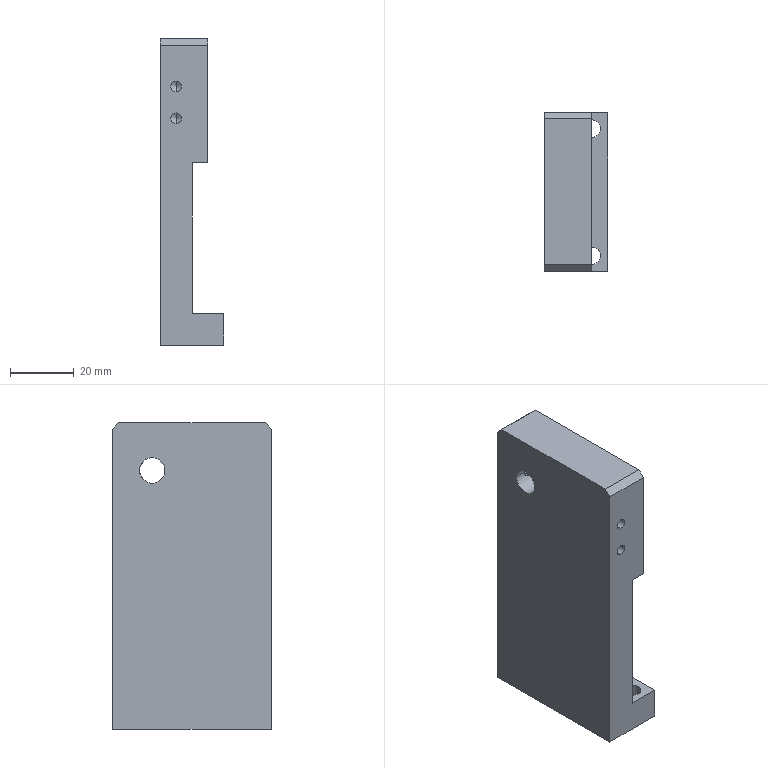Part | STEP file | 11-FG-B00911 | 1 solid | 32 faces | box 20 x 50 x 96.4 mm | volume 61320 mm3 | cylinder 14 | plane 12 | cone 6 | commonest cylinder face diameters 3.3 x8 5.5 x4 8 x2
STEP:
#1=CARTESIAN_POINT('',(17.75,5.,-7.4));
#2=VERTEX_POINT('',#1);
#3=CARTESIAN_POINT('',(12.25,5.,-7.4));
#4=VERTEX_POINT('',#3);
#5=CARTESIAN_POINT('',(15.,5.,-7.4));
#6=DIRECTION('',(0.,0.,-1.));
#7=DIRECTION('',(1.,0.,0.));
#8=AXIS2_PLACEMENT_3D('',#5,#6,#7);
#9=CIRCLE('',#8,2.75);
#10=EDGE_CURVE('',#2,#4,#9,.T.);
#11=ORIENTED_EDGE('',*,*,#10,.T.);
#12=CARTESIAN_POINT('',(12.25,5.,2.6));
#13=VERTEX_POINT('',#12);
#14=CARTESIAN_POINT('',(12.25,5.,-7.4));
#15=DIRECTION('',(0.,0.,1.));
#16=VECTOR('',#15,1000.);
#17=LINE('',#14,#16);
#18=EDGE_CURVE('',#4,#13,#17,.T.);
#19=ORIENTED_EDGE('',*,*,#18,.T.);
#20=CARTESIAN_POINT('',(17.75,5.,2.6));
#21=VERTEX_POINT('',#20);
#22=CARTESIAN_POINT('',(15.,5.,2.6));
#23=DIRECTION('',(0.,0.,1.));
#24=DIRECTION('',(-1.,0.,0.));
#25=AXIS2_PLACEMENT_3D('',#22,#23,#24);
#26=CIRCLE('',#25,2.75);
#27=EDGE_CURVE('',#13,#21,#26,.T.);
#28=ORIENTED_EDGE('',*,*,#27,.T.);
#29=CARTESIAN_POINT('',(17.75,5.,-7.4));
#30=DIRECTION('',(0.,0.,1.));
#31=VECTOR('',#30,1000.);
#32=LINE('',#29,#31);
#33=EDGE_CURVE('',#2,#21,#32,.T.);
#34=ORIENTED_EDGE('',*,*,#33,.F.);
#35=EDGE_LOOP('',(#11,#19,#28,#34));
#36=FACE_OUTER_BOUND('',#35,.T.);
#37=CARTESIAN_POINT('',(15.,5.,-7.4));
#38=DIRECTION('',(0.,0.,1.));
#39=DIRECTION('',(1.,0.,0.));
#40=AXIS2_PLACEMENT_3D('',#37,#38,#39);
#41=CYLINDRICAL_SURFACE('',#40,2.75);
#42=ADVANCED_FACE('',(#36),#41,.F.);
#43=CARTESIAN_POINT('',(5.,10.1,65.65));
#44=VERTEX_POINT('',#43);
#45=CARTESIAN_POINT('',(5.,10.1,62.35));
#46=VERTEX_POINT('',#45);
#47=CARTESIAN_POINT('',(5.,10.1,64.));
#48=DIRECTION('',(0.,-1.,0.));
#49=DIRECTION('',(0.,0.,-1.));
#50=AXIS2_PLACEMENT_3D('',#47,#48,#49);
#51=CIRCLE('',#50,1.65);
#52=EDGE_CURVE('',#44,#46,#51,.T.);
#53=ORIENTED_EDGE('',*,*,#52,.F.);
#54=CARTESIAN_POINT('',(5.,0.,65.65));
#55=VERTEX_POINT('',#54);
#56=CARTESIAN_POINT('',(5.,0.,65.65));
#57=DIRECTION('',(0.,-1.,0.));
#58=VECTOR('',#57,1000.);
#59=LINE('',#56,#58);
#60=EDGE_CURVE('',#44,#55,#59,.T.);
#61=ORIENTED_EDGE('',*,*,#60,.T.);
#62=CARTESIAN_POINT('',(5.,0.,62.35));
#63=VERTEX_POINT('',#62);
#64=CARTESIAN_POINT('',(5.,0.,64.));
#65=DIRECTION('',(0.,-1.,0.));
#66=DIRECTION('',(0.,0.,-1.));
#67=AXIS2_PLACEMENT_3D('',#64,#65,#66);
#68=CIRCLE('',#67,1.65);
#69=EDGE_CURVE('',#55,#63,#68,.T.);
#70=ORIENTED_EDGE('',*,*,#69,.T.);
#71=CARTESIAN_POINT('',(5.,0.,62.35));
#72=DIRECTION('',(0.,-1.,0.));
#73=VECTOR('',#72,1000.);
#74=LINE('',#71,#73);
#75=EDGE_CURVE('',#46,#63,#74,.T.);
#76=ORIENTED_EDGE('',*,*,#75,.F.);
#77=EDGE_LOOP('',(#53,#61,#70,#76));
#78=FACE_OUTER_BOUND('',#77,.T.);
#79=CARTESIAN_POINT('',(5.,0.,64.));
#80=DIRECTION('',(0.,-1.,0.));
#81=DIRECTION('',(0.,0.,-1.));
#82=AXIS2_PLACEMENT_3D('',#79,#80,#81);
#83=CYLINDRICAL_SURFACE('',#82,1.65);
#84=ADVANCED_FACE('',(#78),#83,.F.);
#85=CARTESIAN_POINT('',(5.,11.091,64.));
#86=VERTEX_POINT('',#85);
#87=CARTESIAN_POINT('',(5.,10.1,62.35));
#88=DIRECTION('',(0.,-0.515,-0.8572));
#89=VECTOR('',#88,1000.);
#90=LINE('',#87,#89);
#91=EDGE_CURVE('',#86,#46,#90,.T.);
#92=ORIENTED_EDGE('',*,*,#91,.F.);
#93=CARTESIAN_POINT('',(5.,10.1,65.65));
#94=DIRECTION('',(0.,-0.515,0.8572));
#95=VECTOR('',#94,1000.);
#96=LINE('',#93,#95);
#97=EDGE_CURVE('',#86,#44,#96,.T.);
#98=ORIENTED_EDGE('',*,*,#97,.T.);
#99=ORIENTED_EDGE('',*,*,#52,.T.);
#100=EDGE_LOOP('',(#92,#98,#99));
#101=FACE_OUTER_BOUND('',#100,.T.);
#102=CARTESIAN_POINT('',(5.,10.1,64.));
#103=DIRECTION('',(0.,-1.,0.));
#104=DIRECTION('',(0.,0.,-1.));
#105=AXIS2_PLACEMENT_3D('',#102,#103,#104);
#106=CONICAL_SURFACE('',#105,1.65,1.03);
#107=ADVANCED_FACE('',(#101),#106,.F.);
#108=CARTESIAN_POINT('',(5.,10.1,75.65));
#109=VERTEX_POINT('',#108);
#110=CARTESIAN_POINT('',(5.,10.1,72.35));
#111=VERTEX_POINT('',#110);
#112=CARTESIAN_POINT('',(5.,10.1,74.));
#113=DIRECTION('',(0.,-1.,0.));
#114=DIRECTION('',(0.,0.,-1.));
#115=AXIS2_PLACEMENT_3D('',#112,#113,#114);
#116=CIRCLE('',#115,1.65);
#117=EDGE_CURVE('',#109,#111,#116,.T.);
#118=ORIENTED_EDGE('',*,*,#117,.F.);
#119=CARTESIAN_POINT('',(5.,0.,75.65));
#120=VERTEX_POINT('',#119);
#121=CARTESIAN_POINT('',(5.,0.,75.65));
#122=DIRECTION('',(0.,-1.,0.));
#123=VECTOR('',#122,1000.);
#124=LINE('',#121,#123);
#125=EDGE_CURVE('',#109,#120,#124,.T.);
#126=ORIENTED_EDGE('',*,*,#125,.T.);
#127=CARTESIAN_POINT('',(5.,0.,72.35));
#128=VERTEX_POINT('',#127);
#129=CARTESIAN_POINT('',(5.,0.,74.));
#130=DIRECTION('',(0.,-1.,0.));
#131=DIRECTION('',(0.,0.,-1.));
#132=AXIS2_PLACEMENT_3D('',#129,#130,#131);
#133=CIRCLE('',#132,1.65);
#134=EDGE_CURVE('',#120,#128,#133,.T.);
#135=ORIENTED_EDGE('',*,*,#134,.T.);
#136=CARTESIAN_POINT('',(5.,0.,72.35));
#137=DIRECTION('',(0.,-1.,0.));
#138=VECTOR('',#137,1000.);
#139=LINE('',#136,#138);
#140=EDGE_CURVE('',#111,#128,#139,.T.);
#141=ORIENTED_EDGE('',*,*,#140,.F.);
#142=EDGE_LOOP('',(#118,#126,#135,#141));
#143=FACE_OUTER_BOUND('',#142,.T.);
#144=CARTESIAN_POINT('',(5.,0.,74.));
#145=DIRECTION('',(0.,-1.,0.));
#146=DIRECTION('',(0.,0.,-1.));
#147=AXIS2_PLACEMENT_3D('',#144,#145,#146);
#148=CYLINDRICAL_SURFACE('',#147,1.65);
#149=ADVANCED_FACE('',(#143),#148,.F.);
#150=CARTESIAN_POINT('',(5.,11.091,74.));
#151=VERTEX_POINT('',#150);
#152=CARTESIAN_POINT('',(5.,10.1,72.35));
#153=DIRECTION('',(0.,-0.515,-0.8572));
#154=VECTOR('',#153,1000.);
#155=LINE('',#152,#154);
#156=EDGE_CURVE('',#151,#111,#155,.T.);
#157=ORIENTED_EDGE('',*,*,#156,.F.);
#158=CARTESIAN_POINT('',(5.,10.1,75.65));
#159=DIRECTION('',(0.,-0.515,0.8572));
#160=VECTOR('',#159,1000.);
#161=LINE('',#158,#160);
#162=EDGE_CURVE('',#151,#109,#161,.T.);
#163=ORIENTED_EDGE('',*,*,#162,.T.);
#164=ORIENTED_EDGE('',*,*,#117,.T.);
#165=EDGE_LOOP('',(#157,#163,#164));
#166=FACE_OUTER_BOUND('',#165,.T.);
#167=CARTESIAN_POINT('',(5.,10.1,74.));
#168=DIRECTION('',(0.,-1.,0.));
#169=DIRECTION('',(0.,0.,-1.));
#170=AXIS2_PLACEMENT_3D('',#167,#168,#169);
#171=CONICAL_SURFACE('',#170,1.65,1.03);
#172=ADVANCED_FACE('',(#166),#171,.F.);
#173=CARTESIAN_POINT('',(12.25,45.,-7.4));
#174=VERTEX_POINT('',#173);
#175=CARTESIAN_POINT('',(17.75,45.,-7.4));
#176=VERTEX_POINT('',#175);
#177=CARTESIAN_POINT('',(15.,45.,-7.4));
#178=DIRECTION('',(0.,0.,1.));
#179=DIRECTION('',(1.,0.,0.));
#180=AXIS2_PLACEMENT_3D('',#177,#178,#179);
#181=CIRCLE('',#180,2.75);
#182=EDGE_CURVE('',#174,#176,#181,.T.);
#183=ORIENTED_EDGE('',*,*,#182,.F.);
#184=CARTESIAN_POINT('',(12.25,45.,2.6));
#185=VERTEX_POINT('',#184);
#186=CARTESIAN_POINT('',(12.25,45.,0.));
#187=DIRECTION('',(0.,0.,1.));
#188=VECTOR('',#187,1000.);
#189=LINE('',#186,#188);
#190=EDGE_CURVE('',#174,#185,#189,.T.);
#191=ORIENTED_EDGE('',*,*,#190,.T.);
#192=CARTESIAN_POINT('',(17.75,45.,2.6));
#193=VERTEX_POINT('',#192);
#194=CARTESIAN_POINT('',(15.,45.,2.6));
#195=DIRECTION('',(0.,0.,1.));
#196=DIRECTION('',(1.,0.,0.));
#197=AXIS2_PLACEMENT_3D('',#194,#195,#196);
#198=CIRCLE('',#197,2.75);
#199=EDGE_CURVE('',#185,#193,#198,.T.);
#200=ORIENTED_EDGE('',*,*,#199,.T.);
#201=CARTESIAN_POINT('',(17.75,45.,0.));
#202=DIRECTION('',(0.,0.,1.));
#203=VECTOR('',#202,1000.);
#204=LINE('',#201,#203);
#205=EDGE_CURVE('',#176,#193,#204,.T.);
#206=ORIENTED_EDGE('',*,*,#205,.F.);
#207=EDGE_LOOP('',(#183,#191,#200,#206));
#208=FACE_OUTER_BOUND('',#207,.T.);
#209=CARTESIAN_POINT('',(15.,45.,0.));
#210=DIRECTION('',(0.,0.,1.));
#211=DIRECTION('',(1.,0.,0.));
#212=AXIS2_PLACEMENT_3D('',#209,#210,#211);
#213=CYLINDRICAL_SURFACE('',#212,2.75);
#214=ADVANCED_FACE('',(#208),#213,.F.);
#215=CARTESIAN_POINT('',(5.,41.144,72.35));
#216=VERTEX_POINT('',#215);
#217=CARTESIAN_POINT('',(3.35,41.5,74.));
#218=VERTEX_POINT('',#217);
#219=CARTESIAN_POINT('',(5.,41.144,72.35));
#220=CARTESIAN_POINT('',(4.891,41.144,72.35));
#221=CARTESIAN_POINT('',(4.781,41.149,72.361));
#222=CARTESIAN_POINT('',(4.568,41.168,72.404));
#223=CARTESIAN_POINT('',(4.464,41.182,72.436));
#224=CARTESIAN_POINT('',(4.165,41.233,72.561));
#225=CARTESIAN_POINT('',(3.985,41.28,72.682));
#226=CARTESIAN_POINT('',(3.757,41.349,72.91));
#227=CARTESIAN_POINT('',(3.689,41.372,72.992));
#228=CARTESIAN_POINT('',(3.571,41.414,73.169));
#229=CARTESIAN_POINT('',(3.519,41.433,73.265));
#230=CARTESIAN_POINT('',(3.436,41.465,73.465));
#231=CARTESIAN_POINT('',(3.404,41.478,73.568));
#232=CARTESIAN_POINT('',(3.361,41.495,73.781));
#233=CARTESIAN_POINT('',(3.35,41.5,73.891));
#234=CARTESIAN_POINT('',(3.35,41.5,74.));
#235=B_SPLINE_CURVE_WITH_KNOTS('',3,(#219,#220,#221,#222,#223,#224,#225,#226,#227,#228,#229,#230,#231,#232,#233,#234),.UNSPECIFIED.,.F.,.F.,(4,2,2,2,2,2,2,4),(0.005217,0.005543,0.005869,0.006521,0.006847,0.007172,0.007498,0.007824),.UNSPECIFIED.);
#236=EDGE_CURVE('',#216,#218,#235,.T.);
#237=ORIENTED_EDGE('',*,*,#236,.F.);
#238=CARTESIAN_POINT('',(5.,50.,72.35));
#239=VERTEX_POINT('',#238);
#240=CARTESIAN_POINT('',(5.,50.,72.35));
#241=DIRECTION('',(0.,1.,0.));
#242=VECTOR('',#241,1000.);
#243=LINE('',#240,#242);
#244=EDGE_CURVE('',#216,#239,#243,.T.);
#245=ORIENTED_EDGE('',*,*,#244,.T.);
#246=CARTESIAN_POINT('',(5.,50.,75.65));
#247=VERTEX_POINT('',#246);
#248=CARTESIAN_POINT('',(5.,50.,74.));
#249=DIRECTION('',(0.,1.,0.));
#250=DIRECTION('',(0.,0.,1.));
#251=AXIS2_PLACEMENT_3D('',#248,#249,#250);
#252=CIRCLE('',#251,1.65);
#253=EDGE_CURVE('',#239,#247,#252,.T.);
#254=ORIENTED_EDGE('',*,*,#253,.T.);
#255=CARTESIAN_POINT('',(5.,41.144,75.65));
#256=VERTEX_POINT('',#255);
#257=CARTESIAN_POINT('',(5.,50.,75.65));
#258=DIRECTION('',(0.,1.,0.));
#259=VECTOR('',#258,1000.);
#260=LINE('',#257,#259);
#261=EDGE_CURVE('',#256,#247,#260,.T.);
#262=ORIENTED_EDGE('',*,*,#261,.F.);
#263=CARTESIAN_POINT('',(3.35,41.5,74.));
#264=CARTESIAN_POINT('',(3.35,41.5,74.218));
#265=CARTESIAN_POINT('',(3.394,41.481,74.437));
#266=CARTESIAN_POINT('',(3.519,41.433,74.735));
#267=CARTESIAN_POINT('',(3.571,41.414,74.831));
#268=CARTESIAN_POINT('',(3.69,41.372,75.009));
#269=CARTESIAN_POINT('',(3.758,41.349,75.091));
#270=CARTESIAN_POINT('',(3.909,41.303,75.243));
#271=CARTESIAN_POINT('',(3.993,41.279,75.311));
#272=CARTESIAN_POINT('',(4.17,41.236,75.43));
#273=CARTESIAN_POINT('',(4.264,41.216,75.481));
#274=CARTESIAN_POINT('',(4.565,41.164,75.607));
#275=CARTESIAN_POINT('',(4.779,41.144,75.65));
#276=CARTESIAN_POINT('',(5.,41.144,75.65));
#277=B_SPLINE_CURVE_WITH_KNOTS('',3,(#263,#264,#265,#266,#267,#268,#269,#270,#271,#272,#273,#274,#275,#276),.UNSPECIFIED.,.F.,.F.,(4,2,2,2,2,2,4),(0.007824,0.008476,0.008802,0.009127,0.009453,0.009779,0.01043),.UNSPECIFIED.);
#278=EDGE_CURVE('',#218,#256,#277,.T.);
#279=ORIENTED_EDGE('',*,*,#278,.F.);
#280=EDGE_LOOP('',(#237,#245,#254,#262,#279));
#281=FACE_OUTER_BOUND('',#280,.T.);
#282=CARTESIAN_POINT('',(5.,50.,74.));
#283=DIRECTION('',(0.,1.,0.));
#284=DIRECTION('',(0.,0.,1.));
#285=AXIS2_PLACEMENT_3D('',#282,#283,#284);
#286=CYLINDRICAL_SURFACE('',#285,1.65);
#287=ADVANCED_FACE('',(#281),#286,.F.);
#288=CARTESIAN_POINT('',(5.,39.9,62.35));
#289=VERTEX_POINT('',#288);
#290=CARTESIAN_POINT('',(5.,39.9,65.65));
#291=VERTEX_POINT('',#290);
#292=CARTESIAN_POINT('',(5.,39.9,64.));
#293=DIRECTION('',(0.,1.,0.));
#294=DIRECTION('',(0.,0.,1.));
#295=AXIS2_PLACEMENT_3D('',#292,#293,#294);
#296=CIRCLE('',#295,1.65);
#297=EDGE_CURVE('',#289,#291,#296,.T.);
#298=ORIENTED_EDGE('',*,*,#297,.F.);
#299=CARTESIAN_POINT('',(5.,50.,62.35));
#300=VERTEX_POINT('',#299);
#301=CARTESIAN_POINT('',(5.,50.,62.35));
#302=DIRECTION('',(0.,1.,0.));
#303=VECTOR('',#302,1000.);
#304=LINE('',#301,#303);
#305=EDGE_CURVE('',#289,#300,#304,.T.);
#306=ORIENTED_EDGE('',*,*,#305,.T.);
#307=CARTESIAN_POINT('',(5.,50.,65.65));
#308=VERTEX_POINT('',#307);
#309=CARTESIAN_POINT('',(5.,50.,64.));
#310=DIRECTION('',(0.,1.,0.));
#311=DIRECTION('',(0.,0.,1.));
#312=AXIS2_PLACEMENT_3D('',#309,#310,#311);
#313=CIRCLE('',#312,1.65);
#314=EDGE_CURVE('',#300,#308,#313,.T.);
#315=ORIENTED_EDGE('',*,*,#314,.T.);
#316=CARTESIAN_POINT('',(5.,50.,65.65));
#317=DIRECTION('',(0.,1.,0.));
#318=VECTOR('',#317,1000.);
#319=LINE('',#316,#318);
#320=EDGE_CURVE('',#291,#308,#319,.T.);
#321=ORIENTED_EDGE('',*,*,#320,.F.);
#322=EDGE_LOOP('',(#298,#306,#315,#321));
#323=FACE_OUTER_BOUND('',#322,.T.);
#324=CARTESIAN_POINT('',(5.,50.,64.));
#325=DIRECTION('',(0.,1.,0.));
#326=DIRECTION('',(0.,0.,1.));
#327=AXIS2_PLACEMENT_3D('',#324,#325,#326);
#328=CYLINDRICAL_SURFACE('',#327,1.65);
#329=ADVANCED_FACE('',(#323),#328,.F.);
#330=CARTESIAN_POINT('',(5.,38.909,64.));
#331=VERTEX_POINT('',#330);
#332=CARTESIAN_POINT('',(5.,39.9,65.65));
#333=DIRECTION('',(0.,0.515,0.8572));
#334=VECTOR('',#333,1000.);
#335=LINE('',#332,#334);
#336=EDGE_CURVE('',#331,#291,#335,.T.);
#337=ORIENTED_EDGE('',*,*,#336,.F.);
#338=CARTESIAN_POINT('',(5.,39.9,62.35));
#339=DIRECTION('',(0.,0.515,-0.8572));
#340=VECTOR('',#339,1000.);
#341=LINE('',#338,#340);
#342=EDGE_CURVE('',#331,#289,#341,.T.);
#343=ORIENTED_EDGE('',*,*,#342,.T.);
#344=ORIENTED_EDGE('',*,*,#297,.T.);
#345=EDGE_LOOP('',(#337,#343,#344));
#346=FACE_OUTER_BOUND('',#345,.T.);
#347=CARTESIAN_POINT('',(5.,39.9,64.));
#348=DIRECTION('',(0.,1.,0.));
#349=DIRECTION('',(0.,0.,1.));
#350=AXIS2_PLACEMENT_3D('',#347,#348,#349);
#351=CONICAL_SURFACE('',#350,1.65,1.03);
#352=ADVANCED_FACE('',(#346),#351,.F.);
#353=CARTESIAN_POINT('',(15.,41.5,74.));
#354=VERTEX_POINT('',#353);
#355=CARTESIAN_POINT('',(15.,33.5,74.));
#356=VERTEX_POINT('',#355);
#357=CARTESIAN_POINT('',(15.,37.5,74.));
#358=DIRECTION('',(-1.,0.,0.));
#359=DIRECTION('',(0.,-1.,0.));
#360=AXIS2_PLACEMENT_3D('',#357,#358,#359);
#361=CIRCLE('',#360,4.);
#362=EDGE_CURVE('',#354,#356,#361,.T.);
#363=ORIENTED_EDGE('',*,*,#362,.F.);
#364=CARTESIAN_POINT('',(6.65,41.5,74.));
#365=VERTEX_POINT('',#364);
#366=CARTESIAN_POINT('',(20.,41.5,74.));
#367=DIRECTION('',(-1.,0.,0.));
#368=VECTOR('',#367,1000.);
#369=LINE('',#366,#368);
#370=EDGE_CURVE('',#354,#365,#369,.T.);
#371=ORIENTED_EDGE('',*,*,#370,.T.);
#372=CARTESIAN_POINT('',(6.65,41.5,74.));
#373=CARTESIAN_POINT('',(6.65,41.5,73.891));
#374=CARTESIAN_POINT('',(6.639,41.495,73.78));
#375=CARTESIAN_POINT('',(6.596,41.478,73.568));
#376=CARTESIAN_POINT('',(6.564,41.465,73.464));
#377=CARTESIAN_POINT('',(6.48,41.433,73.263));
#378=CARTESIAN_POINT('',(6.429,41.414,73.168));
#379=CARTESIAN_POINT('',(6.31,41.372,72.991));
#380=CARTESIAN_POINT('',(6.241,41.349,72.907));
#381=CARTESIAN_POINT('',(6.09,41.303,72.756));
#382=CARTESIAN_POINT('',(6.008,41.28,72.689));
#383=CARTESIAN_POINT('',(5.829,41.236,72.57));
#384=CARTESIAN_POINT('',(5.734,41.216,72.518));
#385=CARTESIAN_POINT('',(5.437,41.165,72.394));
#386=CARTESIAN_POINT('',(5.217,41.144,72.35));
#387=CARTESIAN_POINT('',(5.,41.144,72.35));
#388=B_SPLINE_CURVE_WITH_KNOTS('',3,(#372,#373,#374,#375,#376,#377,#378,#379,#380,#381,#382,#383,#384,#385,#386,#387),.UNSPECIFIED.,.F.,.F.,(4,2,2,2,2,2,2,4),(0.00261,0.002935,0.003261,0.003587,0.003913,0.004239,0.004565,0.005217),.UNSPECIFIED.);
#389=EDGE_CURVE('',#365,#216,#388,.T.);
#390=ORIENTED_EDGE('',*,*,#389,.T.);
#391=ORIENTED_EDGE('',*,*,#236,.T.);
#392=CARTESIAN_POINT('',(0.,41.5,74.));
#393=VERTEX_POINT('',#392);
#394=CARTESIAN_POINT('',(20.,41.5,74.));
#395=DIRECTION('',(-1.,0.,0.));
#396=VECTOR('',#395,1000.);
#397=LINE('',#394,#396);
#398=EDGE_CURVE('',#218,#393,#397,.T.);
#399=ORIENTED_EDGE('',*,*,#398,.T.);
#400=CARTESIAN_POINT('',(0.,33.5,74.));
#401=VERTEX_POINT('',#400);
#402=CARTESIAN_POINT('',(0.,37.5,74.));
#403=DIRECTION('',(-1.,0.,0.));
#404=DIRECTION('',(0.,-1.,0.));
#405=AXIS2_PLACEMENT_3D('',#402,#403,#404);
#406=CIRCLE('',#405,4.);
#407=EDGE_CURVE('',#393,#401,#406,.T.);
#408=ORIENTED_EDGE('',*,*,#407,.T.);
#409=CARTESIAN_POINT('',(20.,33.5,74.));
#410=DIRECTION('',(-1.,0.,0.));
#411=VECTOR('',#410,1000.);
#412=LINE('',#409,#411);
#413=EDGE_CURVE('',#356,#401,#412,.T.);
#414=ORIENTED_EDGE('',*,*,#413,.F.);
#415=EDGE_LOOP('',(#363,#371,#390,#391,#399,#408,#414));
#416=FACE_OUTER_BOUND('',#415,.T.);
#417=CARTESIAN_POINT('',(20.,37.5,74.));
#418=DIRECTION('',(-1.,0.,0.));
#419=DIRECTION('',(0.,-1.,0.));
#420=AXIS2_PLACEMENT_3D('',#417,#418,#419);
#421=CYLINDRICAL_SURFACE('',#420,4.);
#422=ADVANCED_FACE('',(#416),#421,.F.);
#423=CARTESIAN_POINT('',(0.,50.,-7.4));
#424=VERTEX_POINT('',#423);
#425=CARTESIAN_POINT('',(0.,0.,-7.4));
#426=VERTEX_POINT('',#425);
#427=CARTESIAN_POINT('',(0.,0.,-7.4));
#428=DIRECTION('',(0.,-1.,0.));
#429=VECTOR('',#428,1000.);
#430=LINE('',#427,#429);
#431=EDGE_CURVE('',#424,#426,#430,.T.);
#432=ORIENTED_EDGE('',*,*,#431,.F.);
#433=CARTESIAN_POINT('',(20.,50.,-7.4));
#434=VERTEX_POINT('',#433);
#435=CARTESIAN_POINT('',(0.,50.,-7.4));
#436=DIRECTION('',(-1.,0.,0.));
#437=VECTOR('',#436,1000.);
#438=LINE('',#435,#437);
#439=EDGE_CURVE('',#434,#424,#438,.T.);
#440=ORIENTED_EDGE('',*,*,#439,.F.);
#441=CARTESIAN_POINT('',(20.,0.,-7.4));
#442=VERTEX_POINT('',#441);
#443=CARTESIAN_POINT('',(20.,0.,-7.4));
#444=DIRECTION('',(0.,1.,0.));
#445=VECTOR('',#444,1000.);
#446=LINE('',#443,#445);
#447=EDGE_CURVE('',#442,#434,#446,.T.);
#448=ORIENTED_EDGE('',*,*,#447,.F.);
#449=CARTESIAN_POINT('',(0.,0.,-7.4));
#450=DIRECTION('',(1.,0.,0.));
#451=VECTOR('',#450,1000.);
#452=LINE('',#449,#451);
#453=EDGE_CURVE('',#426,#442,#452,.T.);
#454=ORIENTED_EDGE('',*,*,#453,.F.);
#455=EDGE_LOOP('',(#432,#440,#448,#454));
#456=FACE_OUTER_BOUND('',#455,.T.);
#457=CARTESIAN_POINT('',(15.,45.,-7.4));
#458=DIRECTION('',(0.,0.,1.));
#459=DIRECTION('',(1.,0.,0.));
#460=AXIS2_PLACEMENT_3D('',#457,#458,#459);
#461=CIRCLE('',#460,2.75);
#462=EDGE_CURVE('',#176,#174,#461,.T.);
#463=ORIENTED_EDGE('',*,*,#462,.T.);
#464=ORIENTED_EDGE('',*,*,#182,.T.);
#465=EDGE_LOOP('',(#463,#464));
#466=FACE_BOUND('',#465,.T.);
#467=ORIENTED_EDGE('',*,*,#10,.F.);
#468=CARTESIAN_POINT('',(15.,5.,-7.4));
#469=DIRECTION('',(0.,0.,-1.));
#470=DIRECTION('',(1.,0.,0.));
#471=AXIS2_PLACEMENT_3D('',#468,#469,#470);
#472=CIRCLE('',#471,2.75);
#473=EDGE_CURVE('',#4,#2,#472,.T.);
#474=ORIENTED_EDGE('',*,*,#473,.F.);
#475=EDGE_LOOP('',(#467,#474));
#476=FACE_BOUND('',#475,.T.);
#477=CARTESIAN_POINT('',(0.,50.,-7.4));
#478=DIRECTION('',(0.,0.,-1.));
#479=DIRECTION('',(-1.,0.,0.));
#480=AXIS2_PLACEMENT_3D('',#477,#478,#479);
#481=PLANE('',#480);
#482=ADVANCED_FACE('',(#456,#466,#476),#481,.T.);
#483=CARTESIAN_POINT('',(15.,45.,2.6));
#484=DIRECTION('',(0.,0.,1.));
#485=DIRECTION('',(1.,0.,0.));
#486=AXIS2_PLACEMENT_3D('',#483,#484,#485);
#487=CIRCLE('',#486,2.75);
#488=EDGE_CURVE('',#193,#185,#487,.T.);
#489=ORIENTED_EDGE('',*,*,#488,.F.);
#490=ORIENTED_EDGE('',*,*,#199,.F.);
#491=EDGE_LOOP('',(#489,#490));
#492=FACE_BOUND('',#491,.T.);
#493=CARTESIAN_POINT('',(10.,50.,2.6));
#494=VERTEX_POINT('',#493);
#495=CARTESIAN_POINT('',(10.,0.,2.6));
#496=VERTEX_POINT('',#495);
#497=CARTESIAN_POINT('',(10.,72.,2.6));
#498=DIRECTION('',(0.,-1.,0.));
#499=VECTOR('',#498,1000.);
#500=LINE('',#497,#499);
#501=EDGE_CURVE('',#494,#496,#500,.T.);
#502=ORIENTED_EDGE('',*,*,#501,.T.);
#503=CARTESIAN_POINT('',(20.,0.,2.6));
#504=VERTEX_POINT('',#503);
#505=CARTESIAN_POINT('',(15.,0.,2.6));
#506=DIRECTION('',(1.,0.,0.));
#507=VECTOR('',#506,1000.);
#508=LINE('',#505,#507);
#509=EDGE_CURVE('',#496,#504,#508,.T.);
#510=ORIENTED_EDGE('',*,*,#509,.T.);
#511=CARTESIAN_POINT('',(20.,50.,2.6));
#512=VERTEX_POINT('',#511);
#513=CARTESIAN_POINT('',(20.,50.,2.6));
#514=DIRECTION('',(0.,-1.,0.));
#515=VECTOR('',#514,1000.);
#516=LINE('',#513,#515);
#517=EDGE_CURVE('',#512,#504,#516,.T.);
#518=ORIENTED_EDGE('',*,*,#517,.F.);
#519=CARTESIAN_POINT('',(0.,50.,2.6));
#520=DIRECTION('',(1.,0.,0.));
#521=VECTOR('',#520,1000.);
#522=LINE('',#519,#521);
#523=EDGE_CURVE('',#494,#512,#522,.T.);
#524=ORIENTED_EDGE('',*,*,#523,.F.);
#525=EDGE_LOOP('',(#502,#510,#518,#524));
#526=FACE_OUTER_BOUND('',#525,.T.);
#527=CARTESIAN_POINT('',(15.,5.,2.6));
#528=DIRECTION('',(0.,0.,1.));
#529=DIRECTION('',(-1.,0.,0.));
#530=AXIS2_PLACEMENT_3D('',#527,#528,#529);
#531=CIRCLE('',#530,2.75);
#532=EDGE_CURVE('',#21,#13,#531,.T.);
#533=ORIENTED_EDGE('',*,*,#532,.F.);
#534=ORIENTED_EDGE('',*,*,#27,.F.);
#535=EDGE_LOOP('',(#533,#534));
#536=FACE_BOUND('',#535,.T.);
#537=CARTESIAN_POINT('',(15.,72.,2.6));
#538=DIRECTION('',(0.,0.,-1.));
#539=DIRECTION('',(-1.,0.,0.));
#540=AXIS2_PLACEMENT_3D('',#537,#538,#539);
#541=PLANE('',#540);
#542=ADVANCED_FACE('',(#492,#526,#536),#541,.F.);
#543=CARTESIAN_POINT('',(0.,37.5,74.));
#544=DIRECTION('',(-1.,0.,0.));
#545=DIRECTION('',(0.,-1.,0.));
#546=AXIS2_PLACEMENT_3D('',#543,#544,#545);
#547=CIRCLE('',#546,4.);
#548=EDGE_CURVE('',#401,#393,#547,.T.);
#549=ORIENTED_EDGE('',*,*,#548,.F.);
#550=ORIENTED_EDGE('',*,*,#407,.F.);
#551=EDGE_LOOP('',(#549,#550));
#552=FACE_BOUND('',#551,.T.);
#553=CARTESIAN_POINT('',(0.,48.,89.));
#554=VERTEX_POINT('',#553);
#555=CARTESIAN_POINT('',(0.,2.,89.));
#556=VERTEX_POINT('',#555);
#557=CARTESIAN_POINT('',(0.,0.,89.));
#558=DIRECTION('',(0.,-1.,0.));
#559=VECTOR('',#558,1000.);
#560=LINE('',#557,#559);
#561=EDGE_CURVE('',#554,#556,#560,.T.);
#562=ORIENTED_EDGE('',*,*,#561,.F.);
#563=CARTESIAN_POINT('',(0.,50.,87.));
#564=VERTEX_POINT('',#563);
#565=CARTESIAN_POINT('',(0.,48.,89.));
#566=DIRECTION('',(0.,0.7071,-0.7071));
#567=VECTOR('',#566,1000.);
#568=LINE('',#565,#567);
#569=EDGE_CURVE('',#554,#564,#568,.T.);
#570=ORIENTED_EDGE('',*,*,#569,.T.);
#571=CARTESIAN_POINT('',(0.,50.,89.));
#572=DIRECTION('',(0.,0.,-1.));
#573=VECTOR('',#572,1000.);
#574=LINE('',#571,#573);
#575=EDGE_CURVE('',#564,#424,#574,.T.);
#576=ORIENTED_EDGE('',*,*,#575,.T.);
#577=ORIENTED_EDGE('',*,*,#431,.T.);
#578=CARTESIAN_POINT('',(0.,0.,87.));
#579=VERTEX_POINT('',#578);
#580=CARTESIAN_POINT('',(0.,0.,89.));
#581=DIRECTION('',(0.,0.,-1.));
#582=VECTOR('',#581,1000.);
#583=LINE('',#580,#582);
#584=EDGE_CURVE('',#579,#426,#583,.T.);
#585=ORIENTED_EDGE('',*,*,#584,.F.);
#586=CARTESIAN_POINT('',(0.,2.,89.));
#587=DIRECTION('',(0.,0.7071,0.7071));
#588=VECTOR('',#587,1000.);
#589=LINE('',#586,#588);
#590=EDGE_CURVE('',#579,#556,#589,.T.);
#591=ORIENTED_EDGE('',*,*,#590,.T.);
#592=EDGE_LOOP('',(#562,#570,#576,#577,#585,#591));
#593=FACE_OUTER_BOUND('',#592,.T.);
#594=CARTESIAN_POINT('',(0.,0.,89.));
#595=DIRECTION('',(1.,0.,0.));
#596=DIRECTION('',(0.,1.,0.));
#597=AXIS2_PLACEMENT_3D('',#594,#595,#596);
#598=PLANE('',#597);
#599=ADVANCED_FACE('',(#552,#593),#598,.F.);
#600=CARTESIAN_POINT('',(5.,0.,64.));
#601=DIRECTION('',(0.,-1.,0.));
#602=DIRECTION('',(0.,0.,-1.));
#603=AXIS2_PLACEMENT_3D('',#600,#601,#602);
#604=CIRCLE('',#603,1.65);
#605=EDGE_CURVE('',#63,#55,#604,.T.);
#606=ORIENTED_EDGE('',*,*,#605,.F.);
#607=ORIENTED_EDGE('',*,*,#69,.F.);
#608=EDGE_LOOP('',(#606,#607));
#609=FACE_BOUND('',#608,.T.);
#610=CARTESIAN_POINT('',(5.,0.,74.));
#611=DIRECTION('',(0.,-1.,0.));
#612=DIRECTION('',(0.,0.,-1.));
#613=AXIS2_PLACEMENT_3D('',#610,#611,#612);
#614=CIRCLE('',#613,1.65);
#615=EDGE_CURVE('',#128,#120,#614,.T.);
#616=ORIENTED_EDGE('',*,*,#615,.F.);
#617=ORIENTED_EDGE('',*,*,#134,.F.);
#618=EDGE_LOOP('',(#616,#617));
#619=FACE_BOUND('',#618,.T.);
#620=CARTESIAN_POINT('',(15.,0.,87.));
#621=VERTEX_POINT('',#620);
#622=CARTESIAN_POINT('',(15.,0.,50.));
#623=VERTEX_POINT('',#622);
#624=CARTESIAN_POINT('',(15.,0.,89.));
#625=DIRECTION('',(0.,0.,-1.));
#626=VECTOR('',#625,1000.);
#627=LINE('',#624,#626);
#628=EDGE_CURVE('',#621,#623,#627,.T.);
#629=ORIENTED_EDGE('',*,*,#628,.F.);
#630=CARTESIAN_POINT('',(0.,0.,87.));
#631=DIRECTION('',(-1.,0.,0.));
#632=VECTOR('',#631,1000.);
#633=LINE('',#630,#632);
#634=EDGE_CURVE('',#621,#579,#633,.T.);
#635=ORIENTED_EDGE('',*,*,#634,.T.);
#636=ORIENTED_EDGE('',*,*,#584,.T.);
#637=ORIENTED_EDGE('',*,*,#453,.T.);
#638=CARTESIAN_POINT('',(20.,0.,10.));
#639=DIRECTION('',(0.,0.,-1.));
#640=VECTOR('',#639,1000.);
#641=LINE('',#638,#640);
#642=EDGE_CURVE('',#504,#442,#641,.T.);
#643=ORIENTED_EDGE('',*,*,#642,.F.);
#644=ORIENTED_EDGE('',*,*,#509,.F.);
#645=CARTESIAN_POINT('',(10.,0.,50.));
#646=VERTEX_POINT('',#645);
#647=CARTESIAN_POINT('',(10.,0.,10.));
#648=DIRECTION('',(0.,0.,-1.));
#649=VECTOR('',#648,1000.);
#650=LINE('',#647,#649);
#651=EDGE_CURVE('',#646,#496,#650,.T.);
#652=ORIENTED_EDGE('',*,*,#651,.F.);
#653=CARTESIAN_POINT('',(15.,0.,50.));
#654=DIRECTION('',(-1.,0.,0.));
#655=VECTOR('',#654,1000.);
#656=LINE('',#653,#655);
#657=EDGE_CURVE('',#623,#646,#656,.T.);
#658=ORIENTED_EDGE('',*,*,#657,.F.);
#659=EDGE_LOOP('',(#629,#635,#636,#637,#643,#644,#652,#658));
#660=FACE_OUTER_BOUND('',#659,.T.);
#661=CARTESIAN_POINT('',(0.,0.,89.));
#662=DIRECTION('',(0.,1.,0.));
#663=DIRECTION('',(0.,0.,1.));
#664=AXIS2_PLACEMENT_3D('',#661,#662,#663);
#665=PLANE('',#664);
#666=ADVANCED_FACE('',(#609,#619,#660),#665,.F.);
#667=CARTESIAN_POINT('',(15.,37.5,74.));
#668=DIRECTION('',(-1.,0.,0.));
#669=DIRECTION('',(0.,-1.,0.));
#670=AXIS2_PLACEMENT_3D('',#667,#668,#669);
#671=CIRCLE('',#670,4.);
#672=EDGE_CURVE('',#356,#354,#671,.T.);
#673=ORIENTED_EDGE('',*,*,#672,.T.);
#674=ORIENTED_EDGE('',*,*,#362,.T.);
#675=EDGE_LOOP('',(#673,#674));
#676=FACE_BOUND('',#675,.T.);
#677=CARTESIAN_POINT('',(15.,50.,87.));
#678=VERTEX_POINT('',#677);
#679=CARTESIAN_POINT('',(15.,50.,50.));
#680=VERTEX_POINT('',#679);
#681=CARTESIAN_POINT('',(15.,50.,89.));
#682=DIRECTION('',(0.,0.,-1.));
#683=VECTOR('',#682,1000.);
#684=LINE('',#681,#683);
#685=EDGE_CURVE('',#678,#680,#684,.T.);
#686=ORIENTED_EDGE('',*,*,#685,.F.);
#687=CARTESIAN_POINT('',(15.,48.,89.));
#688=VERTEX_POINT('',#687);
#689=CARTESIAN_POINT('',(15.,48.,89.));
#690=DIRECTION('',(0.,-0.7071,0.7071));
#691=VECTOR('',#690,1000.);
#692=LINE('',#689,#691);
#693=EDGE_CURVE('',#678,#688,#692,.T.);
#694=ORIENTED_EDGE('',*,*,#693,.T.);
#695=CARTESIAN_POINT('',(15.,2.,89.));
#696=VERTEX_POINT('',#695);
#697=CARTESIAN_POINT('',(15.,0.,89.));
#698=DIRECTION('',(0.,1.,0.));
#699=VECTOR('',#698,1000.);
#700=LINE('',#697,#699);
#701=EDGE_CURVE('',#696,#688,#700,.T.);
#702=ORIENTED_EDGE('',*,*,#701,.F.);
#703=CARTESIAN_POINT('',(15.,2.,89.));
#704=DIRECTION('',(0.,-0.7071,-0.7071));
#705=VECTOR('',#704,1000.);
#706=LINE('',#703,#705);
#707=EDGE_CURVE('',#696,#621,#706,.T.);
#708=ORIENTED_EDGE('',*,*,#707,.T.);
#709=ORIENTED_EDGE('',*,*,#628,.T.);
#710=CARTESIAN_POINT('',(15.,72.,50.));
#711=DIRECTION('',(0.,-1.,0.));
#712=VECTOR('',#711,1000.);
#713=LINE('',#710,#712);
#714=EDGE_CURVE('',#680,#623,#713,.T.);
#715=ORIENTED_EDGE('',*,*,#714,.F.);
#716=EDGE_LOOP('',(#686,#694,#702,#708,#709,#715));
#717=FACE_OUTER_BOUND('',#716,.T.);
#718=CARTESIAN_POINT('',(15.,0.,89.));
#719=DIRECTION('',(-1.,0.,0.));
#720=DIRECTION('',(0.,-1.,0.));
#721=AXIS2_PLACEMENT_3D('',#718,#719,#720);
#722=PLANE('',#721);
#723=ADVANCED_FACE('',(#676,#717),#722,.F.);
#724=CARTESIAN_POINT('',(5.,50.,74.));
#725=DIRECTION('',(0.,1.,0.));
#726=DIRECTION('',(0.,0.,1.));
#727=AXIS2_PLACEMENT_3D('',#724,#725,#726);
#728=CIRCLE('',#727,1.65);
#729=EDGE_CURVE('',#247,#239,#728,.T.);
#730=ORIENTED_EDGE('',*,*,#729,.F.);
#731=ORIENTED_EDGE('',*,*,#253,.F.);
#732=EDGE_LOOP('',(#730,#731));
#733=FACE_BOUND('',#732,.T.);
#734=CARTESIAN_POINT('',(5.,50.,64.));
#735=DIRECTION('',(0.,1.,0.));
#736=DIRECTION('',(0.,0.,1.));
#737=AXIS2_PLACEMENT_3D('',#734,#735,#736);
#738=CIRCLE('',#737,1.65);
#739=EDGE_CURVE('',#308,#300,#738,.T.);
#740=ORIENTED_EDGE('',*,*,#739,.F.);
#741=ORIENTED_EDGE('',*,*,#314,.F.);
#742=EDGE_LOOP('',(#740,#741));
#743=FACE_BOUND('',#742,.T.);
#744=ORIENTED_EDGE('',*,*,#575,.F.);
#745=CARTESIAN_POINT('',(0.,50.,87.));
#746=DIRECTION('',(1.,0.,0.));
#747=VECTOR('',#746,1000.);
#748=LINE('',#745,#747);
#749=EDGE_CURVE('',#564,#678,#748,.T.);
#750=ORIENTED_EDGE('',*,*,#749,.T.);
#751=ORIENTED_EDGE('',*,*,#685,.T.);
#752=CARTESIAN_POINT('',(10.,50.,50.));
#753=VERTEX_POINT('',#752);
#754=CARTESIAN_POINT('',(0.,50.,50.));
#755=DIRECTION('',(-1.,0.,0.));
#756=VECTOR('',#755,1000.);
#757=LINE('',#754,#756);
#758=EDGE_CURVE('',#680,#753,#757,.T.);
#759=ORIENTED_EDGE('',*,*,#758,.T.);
#760=CARTESIAN_POINT('',(10.,50.,89.));
#761=DIRECTION('',(0.,0.,-1.));
#762=VECTOR('',#761,1000.);
#763=LINE('',#760,#762);
#764=EDGE_CURVE('',#753,#494,#763,.T.);
#765=ORIENTED_EDGE('',*,*,#764,.T.);
#766=ORIENTED_EDGE('',*,*,#523,.T.);
#767=CARTESIAN_POINT('',(20.,50.,0.));
#768=DIRECTION('',(0.,0.,1.));
#769=VECTOR('',#768,1000.);
#770=LINE('',#767,#769);
#771=EDGE_CURVE('',#434,#512,#770,.T.);
#772=ORIENTED_EDGE('',*,*,#771,.F.);
#773=ORIENTED_EDGE('',*,*,#439,.T.);
#774=EDGE_LOOP('',(#744,#750,#751,#759,#765,#766,#772,#773));
#775=FACE_OUTER_BOUND('',#774,.T.);
#776=CARTESIAN_POINT('',(0.,50.,89.));
#777=DIRECTION('',(0.,-1.,0.));
#778=DIRECTION('',(0.,0.,-1.));
#779=AXIS2_PLACEMENT_3D('',#776,#777,#778);
#780=PLANE('',#779);
#781=ADVANCED_FACE('',(#733,#743,#775),#780,.F.);
#782=ORIENTED_EDGE('',*,*,#701,.T.);
#783=CARTESIAN_POINT('',(0.,48.,89.));
#784=DIRECTION('',(-1.,0.,0.));
#785=VECTOR('',#784,1000.);
#786=LINE('',#783,#785);
#787=EDGE_CURVE('',#688,#554,#786,.T.);
#788=ORIENTED_EDGE('',*,*,#787,.T.);
#789=ORIENTED_EDGE('',*,*,#561,.T.);
#790=CARTESIAN_POINT('',(0.,2.,89.));
#791=DIRECTION('',(1.,0.,0.));
#792=VECTOR('',#791,1000.);
#793=LINE('',#790,#792);
#794=EDGE_CURVE('',#556,#696,#793,.T.);
#795=ORIENTED_EDGE('',*,*,#794,.T.);
#796=EDGE_LOOP('',(#782,#788,#789,#795));
#797=FACE_OUTER_BOUND('',#796,.T.);
#798=CARTESIAN_POINT('',(0.,50.,89.));
#799=DIRECTION('',(0.,0.,-1.));
#800=DIRECTION('',(-1.,0.,0.));
#801=AXIS2_PLACEMENT_3D('',#798,#799,#800);
#802=PLANE('',#801);
#803=ADVANCED_FACE('',(#797),#802,.F.);
#804=CARTESIAN_POINT('',(10.,72.,50.));
#805=DIRECTION('',(0.,-1.,0.));
#806=VECTOR('',#805,1000.);
#807=LINE('',#804,#806);
#808=EDGE_CURVE('',#753,#646,#807,.T.);
#809=ORIENTED_EDGE('',*,*,#808,.T.);
#810=ORIENTED_EDGE('',*,*,#651,.T.);
#811=ORIENTED_EDGE('',*,*,#501,.F.);
#812=ORIENTED_EDGE('',*,*,#764,.F.);
#813=EDGE_LOOP('',(#809,#810,#811,#812));
#814=FACE_OUTER_BOUND('',#813,.T.);
#815=CARTESIAN_POINT('',(10.,72.,10.));
#816=DIRECTION('',(-1.,0.,0.));
#817=DIRECTION('',(0.,0.,1.));
#818=AXIS2_PLACEMENT_3D('',#815,#816,#817);
#819=PLANE('',#818);
#820=ADVANCED_FACE('',(#814),#819,.F.);
#821=ORIENTED_EDGE('',*,*,#714,.T.);
#822=ORIENTED_EDGE('',*,*,#657,.T.);
#823=ORIENTED_EDGE('',*,*,#808,.F.);
#824=ORIENTED_EDGE('',*,*,#758,.F.);
#825=EDGE_LOOP('',(#821,#822,#823,#824));
#826=FACE_OUTER_BOUND('',#825,.T.);
#827=CARTESIAN_POINT('',(15.,72.,50.));
#828=DIRECTION('',(0.,0.,1.));
#829=DIRECTION('',(1.,0.,0.));
#830=AXIS2_PLACEMENT_3D('',#827,#828,#829);
#831=PLANE('',#830);
#832=ADVANCED_FACE('',(#826),#831,.F.);
#833=ORIENTED_EDGE('',*,*,#447,.T.);
#834=ORIENTED_EDGE('',*,*,#771,.T.);
#835=ORIENTED_EDGE('',*,*,#517,.T.);
#836=ORIENTED_EDGE('',*,*,#642,.T.);
#837=EDGE_LOOP('',(#833,#834,#835,#836));
#838=FACE_OUTER_BOUND('',#837,.T.);
#839=CARTESIAN_POINT('',(20.,50.,0.));
#840=DIRECTION('',(1.,0.,0.));
#841=DIRECTION('',(0.,1.,0.));
#842=AXIS2_PLACEMENT_3D('',#839,#840,#841);
#843=PLANE('',#842);
#844=ADVANCED_FACE('',(#838),#843,.T.);
#845=ORIENTED_EDGE('',*,*,#370,.F.);
#846=ORIENTED_EDGE('',*,*,#672,.F.);
#847=ORIENTED_EDGE('',*,*,#413,.T.);
#848=ORIENTED_EDGE('',*,*,#548,.T.);
#849=ORIENTED_EDGE('',*,*,#398,.F.);
#850=ORIENTED_EDGE('',*,*,#278,.T.);
#851=CARTESIAN_POINT('',(5.,41.144,75.65));
#852=CARTESIAN_POINT('',(5.11,41.144,75.65));
#853=CARTESIAN_POINT('',(5.219,41.149,75.639));
#854=CARTESIAN_POINT('',(5.431,41.168,75.596));
#855=CARTESIAN_POINT('',(5.537,41.182,75.564));
#856=CARTESIAN_POINT('',(5.835,41.233,75.439));
#857=CARTESIAN_POINT('',(6.017,41.28,75.317));
#858=CARTESIAN_POINT('',(6.317,41.372,75.016));
#859=CARTESIAN_POINT('',(6.44,41.417,74.834));
#860=CARTESIAN_POINT('',(6.564,41.465,74.536));
#861=CARTESIAN_POINT('',(6.596,41.478,74.431));
#862=CARTESIAN_POINT('',(6.639,41.496,74.217));
#863=CARTESIAN_POINT('',(6.65,41.5,74.109));
#864=CARTESIAN_POINT('',(6.65,41.5,74.));
#865=B_SPLINE_CURVE_WITH_KNOTS('',3,(#851,#852,#853,#854,#855,#856,#857,#858,#859,#860,#861,#862,#863,#864),.UNSPECIFIED.,.F.,.F.,(4,2,2,2,2,2,4),(0.,0.0003262,0.0006524,0.001305,0.001957,0.002283,0.00261),.UNSPECIFIED.);
#866=EDGE_CURVE('',#256,#365,#865,.T.);
#867=ORIENTED_EDGE('',*,*,#866,.T.);
#868=EDGE_LOOP('',(#845,#846,#847,#848,#849,#850,#867));
#869=FACE_OUTER_BOUND('',#868,.T.);
#870=CARTESIAN_POINT('',(20.,37.5,74.));
#871=DIRECTION('',(-1.,0.,0.));
#872=DIRECTION('',(0.,-1.,0.));
#873=AXIS2_PLACEMENT_3D('',#870,#871,#872);
#874=CYLINDRICAL_SURFACE('',#873,4.);
#875=ADVANCED_FACE('',(#869),#874,.F.);
#876=ORIENTED_EDGE('',*,*,#342,.F.);
#877=ORIENTED_EDGE('',*,*,#336,.T.);
#878=CARTESIAN_POINT('',(5.,39.9,64.));
#879=DIRECTION('',(0.,1.,0.));
#880=DIRECTION('',(0.,0.,1.));
#881=AXIS2_PLACEMENT_3D('',#878,#879,#880);
#882=CIRCLE('',#881,1.65);
#883=EDGE_CURVE('',#291,#289,#882,.T.);
#884=ORIENTED_EDGE('',*,*,#883,.T.);
#885=EDGE_LOOP('',(#876,#877,#884));
#886=FACE_OUTER_BOUND('',#885,.T.);
#887=CARTESIAN_POINT('',(5.,39.9,64.));
#888=DIRECTION('',(0.,1.,0.));
#889=DIRECTION('',(0.,0.,1.));
#890=AXIS2_PLACEMENT_3D('',#887,#888,#889);
#891=CONICAL_SURFACE('',#890,1.65,1.03);
#892=ADVANCED_FACE('',(#886),#891,.F.);
#893=ORIENTED_EDGE('',*,*,#305,.F.);
#894=ORIENTED_EDGE('',*,*,#883,.F.);
#895=ORIENTED_EDGE('',*,*,#320,.T.);
#896=ORIENTED_EDGE('',*,*,#739,.T.);
#897=EDGE_LOOP('',(#893,#894,#895,#896));
#898=FACE_OUTER_BOUND('',#897,.T.);
#899=CARTESIAN_POINT('',(5.,50.,64.));
#900=DIRECTION('',(0.,1.,0.));
#901=DIRECTION('',(0.,0.,1.));
#902=AXIS2_PLACEMENT_3D('',#899,#900,#901);
#903=CYLINDRICAL_SURFACE('',#902,1.65);
#904=ADVANCED_FACE('',(#898),#903,.F.);
#905=ORIENTED_EDGE('',*,*,#244,.F.);
#906=ORIENTED_EDGE('',*,*,#389,.F.);
#907=ORIENTED_EDGE('',*,*,#866,.F.);
#908=ORIENTED_EDGE('',*,*,#261,.T.);
#909=ORIENTED_EDGE('',*,*,#729,.T.);
#910=EDGE_LOOP('',(#905,#906,#907,#908,#909));
#911=FACE_OUTER_BOUND('',#910,.T.);
#912=CARTESIAN_POINT('',(5.,50.,74.));
#913=DIRECTION('',(0.,1.,0.));
#914=DIRECTION('',(0.,0.,1.));
#915=AXIS2_PLACEMENT_3D('',#912,#913,#914);
#916=CYLINDRICAL_SURFACE('',#915,1.65);
#917=ADVANCED_FACE('',(#911),#916,.F.);
#918=ORIENTED_EDGE('',*,*,#190,.F.);
#919=ORIENTED_EDGE('',*,*,#462,.F.);
#920=ORIENTED_EDGE('',*,*,#205,.T.);
#921=ORIENTED_EDGE('',*,*,#488,.T.);
#922=EDGE_LOOP('',(#918,#919,#920,#921));
#923=FACE_OUTER_BOUND('',#922,.T.);
#924=CARTESIAN_POINT('',(15.,45.,0.));
#925=DIRECTION('',(0.,0.,1.));
#926=DIRECTION('',(1.,0.,0.));
#927=AXIS2_PLACEMENT_3D('',#924,#925,#926);
#928=CYLINDRICAL_SURFACE('',#927,2.75);
#929=ADVANCED_FACE('',(#923),#928,.F.);
#930=ORIENTED_EDGE('',*,*,#162,.F.);
#931=ORIENTED_EDGE('',*,*,#156,.T.);
#932=CARTESIAN_POINT('',(5.,10.1,74.));
#933=DIRECTION('',(0.,-1.,0.));
#934=DIRECTION('',(0.,0.,-1.));
#935=AXIS2_PLACEMENT_3D('',#932,#933,#934);
#936=CIRCLE('',#935,1.65);
#937=EDGE_CURVE('',#111,#109,#936,.T.);
#938=ORIENTED_EDGE('',*,*,#937,.T.);
#939=EDGE_LOOP('',(#930,#931,#938));
#940=FACE_OUTER_BOUND('',#939,.T.);
#941=CARTESIAN_POINT('',(5.,10.1,74.));
#942=DIRECTION('',(0.,-1.,0.));
#943=DIRECTION('',(0.,0.,-1.));
#944=AXIS2_PLACEMENT_3D('',#941,#942,#943);
#945=CONICAL_SURFACE('',#944,1.65,1.03);
#946=ADVANCED_FACE('',(#940),#945,.F.);
#947=ORIENTED_EDGE('',*,*,#125,.F.);
#948=ORIENTED_EDGE('',*,*,#937,.F.);
#949=ORIENTED_EDGE('',*,*,#140,.T.);
#950=ORIENTED_EDGE('',*,*,#615,.T.);
#951=EDGE_LOOP('',(#947,#948,#949,#950));
#952=FACE_OUTER_BOUND('',#951,.T.);
#953=CARTESIAN_POINT('',(5.,0.,74.));
#954=DIRECTION('',(0.,-1.,0.));
#955=DIRECTION('',(0.,0.,-1.));
#956=AXIS2_PLACEMENT_3D('',#953,#954,#955);
#957=CYLINDRICAL_SURFACE('',#956,1.65);
#958=ADVANCED_FACE('',(#952),#957,.F.);
#959=ORIENTED_EDGE('',*,*,#97,.F.);
#960=ORIENTED_EDGE('',*,*,#91,.T.);
#961=CARTESIAN_POINT('',(5.,10.1,64.));
#962=DIRECTION('',(0.,-1.,0.));
#963=DIRECTION('',(0.,0.,-1.));
#964=AXIS2_PLACEMENT_3D('',#961,#962,#963);
#965=CIRCLE('',#964,1.65);
#966=EDGE_CURVE('',#46,#44,#965,.T.);
#967=ORIENTED_EDGE('',*,*,#966,.T.);
#968=EDGE_LOOP('',(#959,#960,#967));
#969=FACE_OUTER_BOUND('',#968,.T.);
#970=CARTESIAN_POINT('',(5.,10.1,64.));
#971=DIRECTION('',(0.,-1.,0.));
#972=DIRECTION('',(0.,0.,-1.));
#973=AXIS2_PLACEMENT_3D('',#970,#971,#972);
#974=CONICAL_SURFACE('',#973,1.65,1.03);
#975=ADVANCED_FACE('',(#969),#974,.F.);
#976=ORIENTED_EDGE('',*,*,#60,.F.);
#977=ORIENTED_EDGE('',*,*,#966,.F.);
#978=ORIENTED_EDGE('',*,*,#75,.T.);
#979=ORIENTED_EDGE('',*,*,#605,.T.);
#980=EDGE_LOOP('',(#976,#977,#978,#979));
#981=FACE_OUTER_BOUND('',#980,.T.);
#982=CARTESIAN_POINT('',(5.,0.,64.));
#983=DIRECTION('',(0.,-1.,0.));
#984=DIRECTION('',(0.,0.,-1.));
#985=AXIS2_PLACEMENT_3D('',#982,#983,#984);
#986=CYLINDRICAL_SURFACE('',#985,1.65);
#987=ADVANCED_FACE('',(#981),#986,.F.);
#988=ORIENTED_EDGE('',*,*,#18,.F.);
#989=ORIENTED_EDGE('',*,*,#473,.T.);
#990=ORIENTED_EDGE('',*,*,#33,.T.);
#991=ORIENTED_EDGE('',*,*,#532,.T.);
#992=EDGE_LOOP('',(#988,#989,#990,#991));
#993=FACE_OUTER_BOUND('',#992,.T.);
#994=CARTESIAN_POINT('',(15.,5.,-7.4));
#995=DIRECTION('',(0.,0.,1.));
#996=DIRECTION('',(1.,0.,0.));
#997=AXIS2_PLACEMENT_3D('',#994,#995,#996);
#998=CYLINDRICAL_SURFACE('',#997,2.75);
#999=ADVANCED_FACE('',(#993),#998,.F.);
#1000=ORIENTED_EDGE('',*,*,#693,.F.);
#1001=ORIENTED_EDGE('',*,*,#749,.F.);
#1002=ORIENTED_EDGE('',*,*,#569,.F.);
#1003=ORIENTED_EDGE('',*,*,#787,.F.);
#1004=EDGE_LOOP('',(#1000,#1001,#1002,#1003));
#1005=FACE_OUTER_BOUND('',#1004,.T.);
#1006=CARTESIAN_POINT('',(0.,48.,89.));
#1007=DIRECTION('',(0.,-0.7071,-0.7071));
#1008=DIRECTION('',(-1.,0.,0.));
#1009=AXIS2_PLACEMENT_3D('',#1006,#1007,#1008);
#1010=PLANE('',#1009);
#1011=ADVANCED_FACE('',(#1005),#1010,.F.);
#1012=ORIENTED_EDGE('',*,*,#590,.F.);
#1013=ORIENTED_EDGE('',*,*,#634,.F.);
#1014=ORIENTED_EDGE('',*,*,#707,.F.);
#1015=ORIENTED_EDGE('',*,*,#794,.F.);
#1016=EDGE_LOOP('',(#1012,#1013,#1014,#1015));
#1017=FACE_OUTER_BOUND('',#1016,.T.);
#1018=CARTESIAN_POINT('',(0.,2.,89.));
#1019=DIRECTION('',(0.,0.7071,-0.7071));
#1020=DIRECTION('',(1.,0.,0.));
#1021=AXIS2_PLACEMENT_3D('',#1018,#1019,#1020);
#1022=PLANE('',#1021);
#1023=ADVANCED_FACE('',(#1017),#1022,.F.);
#1024=CLOSED_SHELL('',(#42,#84,#107,#149,#172,#214,#287,#329,#352,#422,#482,#542,#599,#666,#723,#781,#803,#820,#832,#844,#875,#892,#904,#917,#929,#946,#958,#975,#987,#999,#1011,#1023));
#1025=MANIFOLD_SOLID_BREP('',#1024);
#1026=CARTESIAN_POINT('',(0.,0.,0.));
#1027=DIRECTION('',(0.,0.,1.));
#1028=DIRECTION('',(1.,0.,0.));
#1029=AXIS2_PLACEMENT_3D('',#1026,#1027,#1028);
#1030=(LENGTH_UNIT()NAMED_UNIT(*)SI_UNIT(.MILLI.,.METRE.));
#1031=UNCERTAINTY_MEASURE_WITH_UNIT(LENGTH_MEASURE(0.00001),#1030,'','');
#1032=(NAMED_UNIT(*)PLANE_ANGLE_UNIT()SI_UNIT($,.RADIAN.));
#1033=(NAMED_UNIT(*)SI_UNIT($,.STERADIAN.)SOLID_ANGLE_UNIT());
#1034=(GEOMETRIC_REPRESENTATION_CONTEXT(3)GLOBAL_UNCERTAINTY_ASSIGNED_CONTEXT((#1031))GLOBAL_UNIT_ASSIGNED_CONTEXT((#1030,#1032,#1033))REPRESENTATION_CONTEXT('',''));
#1035=ADVANCED_BREP_SHAPE_REPRESENTATION('',(#1025,#1029),#1034);